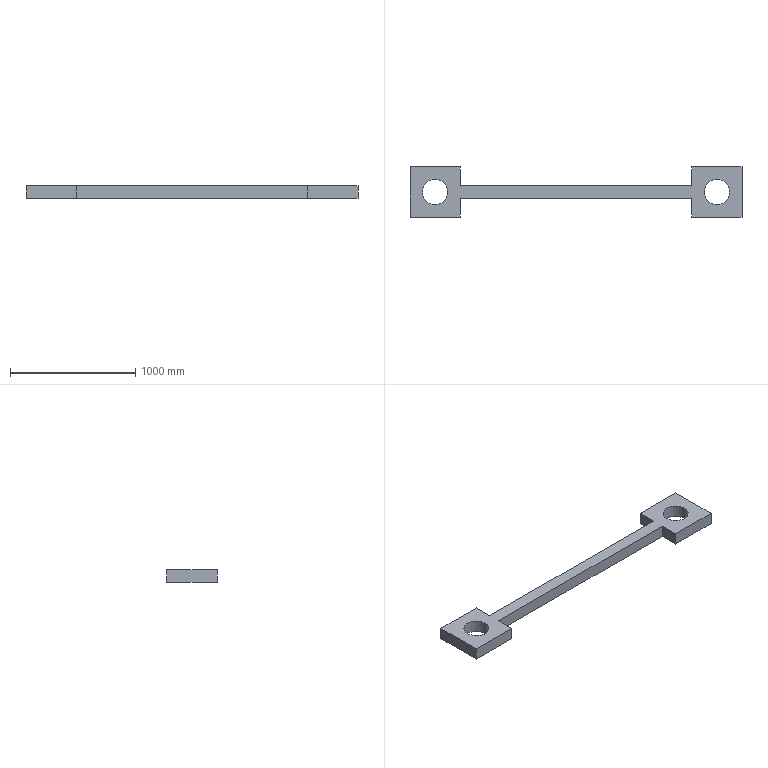Part | SolidWorks | features Extrusion 1 | 1 solid | 18 faces | box 2650 x 400 x 100 mm | volume 44216815 mm3 | plane 14 | cylinder 4 | commonest cylinder face diameters 200 x4
STEP:
#1=CARTESIAN_POINT('',(2150.,0.,100.));
#2=VERTEX_POINT('',#1);
#3=CARTESIAN_POINT('',(2350.,0.,100.));
#4=VERTEX_POINT('',#3);
#5=CARTESIAN_POINT('',(2250.,0.,100.));
#6=DIRECTION('',(0.,0.,1.));
#7=DIRECTION('',(1.,0.,0.));
#8=AXIS2_PLACEMENT_3D('',#5,#6,#7);
#9=CIRCLE('',#8,100.);
#10=EDGE_CURVE('',#2,#4,#9,.T.);
#11=ORIENTED_EDGE('',*,*,#10,.T.);
#12=CARTESIAN_POINT('',(2350.,0.,0.));
#13=VERTEX_POINT('',#12);
#14=CARTESIAN_POINT('',(2350.,0.,100.));
#15=DIRECTION('',(0.,0.,-1.));
#16=VECTOR('',#15,1000.);
#17=LINE('',#14,#16);
#18=EDGE_CURVE('',#4,#13,#17,.T.);
#19=ORIENTED_EDGE('',*,*,#18,.T.);
#20=CARTESIAN_POINT('',(2150.,0.,0.));
#21=VERTEX_POINT('',#20);
#22=CARTESIAN_POINT('',(2250.,0.,0.));
#23=DIRECTION('',(0.,0.,1.));
#24=DIRECTION('',(1.,0.,0.));
#25=AXIS2_PLACEMENT_3D('',#22,#23,#24);
#26=CIRCLE('',#25,100.);
#27=EDGE_CURVE('',#21,#13,#26,.T.);
#28=ORIENTED_EDGE('',*,*,#27,.F.);
#29=CARTESIAN_POINT('',(2150.,0.,100.));
#30=DIRECTION('',(0.,0.,-1.));
#31=VECTOR('',#30,1000.);
#32=LINE('',#29,#31);
#33=EDGE_CURVE('',#2,#21,#32,.T.);
#34=ORIENTED_EDGE('',*,*,#33,.F.);
#35=EDGE_LOOP('',(#11,#19,#28,#34));
#36=FACE_OUTER_BOUND('',#35,.T.);
#37=CARTESIAN_POINT('',(2250.,0.,100.));
#38=DIRECTION('',(0.,0.,-1.));
#39=DIRECTION('',(-1.,0.,0.));
#40=AXIS2_PLACEMENT_3D('',#37,#38,#39);
#41=CYLINDRICAL_SURFACE('',#40,100.);
#42=ADVANCED_FACE('',(#36),#41,.F.);
#43=CARTESIAN_POINT('',(-100.,0.,100.));
#44=VERTEX_POINT('',#43);
#45=CARTESIAN_POINT('',(100.,0.,100.));
#46=VERTEX_POINT('',#45);
#47=CARTESIAN_POINT('',(0.,0.,100.));
#48=DIRECTION('',(0.,0.,1.));
#49=DIRECTION('',(1.,0.,0.));
#50=AXIS2_PLACEMENT_3D('',#47,#48,#49);
#51=CIRCLE('',#50,100.);
#52=EDGE_CURVE('',#44,#46,#51,.T.);
#53=ORIENTED_EDGE('',*,*,#52,.T.);
#54=CARTESIAN_POINT('',(100.,0.,0.));
#55=VERTEX_POINT('',#54);
#56=CARTESIAN_POINT('',(100.,0.,100.));
#57=DIRECTION('',(0.,0.,-1.));
#58=VECTOR('',#57,1000.);
#59=LINE('',#56,#58);
#60=EDGE_CURVE('',#46,#55,#59,.T.);
#61=ORIENTED_EDGE('',*,*,#60,.T.);
#62=CARTESIAN_POINT('',(-100.,0.,0.));
#63=VERTEX_POINT('',#62);
#64=CARTESIAN_POINT('',(0.,0.,0.));
#65=DIRECTION('',(0.,0.,1.));
#66=DIRECTION('',(1.,0.,0.));
#67=AXIS2_PLACEMENT_3D('',#64,#65,#66);
#68=CIRCLE('',#67,100.);
#69=EDGE_CURVE('',#63,#55,#68,.T.);
#70=ORIENTED_EDGE('',*,*,#69,.F.);
#71=CARTESIAN_POINT('',(-100.,0.,100.));
#72=DIRECTION('',(0.,0.,-1.));
#73=VECTOR('',#72,1000.);
#74=LINE('',#71,#73);
#75=EDGE_CURVE('',#44,#63,#74,.T.);
#76=ORIENTED_EDGE('',*,*,#75,.F.);
#77=EDGE_LOOP('',(#53,#61,#70,#76));
#78=FACE_OUTER_BOUND('',#77,.T.);
#79=CARTESIAN_POINT('',(0.,0.,100.));
#80=DIRECTION('',(0.,0.,-1.));
#81=DIRECTION('',(-1.,0.,0.));
#82=AXIS2_PLACEMENT_3D('',#79,#80,#81);
#83=CYLINDRICAL_SURFACE('',#82,100.);
#84=ADVANCED_FACE('',(#78),#83,.F.);
#85=ORIENTED_EDGE('',*,*,#52,.F.);
#86=CARTESIAN_POINT('',(0.,0.,100.));
#87=DIRECTION('',(0.,0.,1.));
#88=DIRECTION('',(1.,0.,0.));
#89=AXIS2_PLACEMENT_3D('',#86,#87,#88);
#90=CIRCLE('',#89,100.);
#91=EDGE_CURVE('',#46,#44,#90,.T.);
#92=ORIENTED_EDGE('',*,*,#91,.F.);
#93=EDGE_LOOP('',(#85,#92));
#94=FACE_BOUND('',#93,.T.);
#95=CARTESIAN_POINT('',(-200.,200.,100.));
#96=VERTEX_POINT('',#95);
#97=CARTESIAN_POINT('',(-200.,-200.,100.));
#98=VERTEX_POINT('',#97);
#99=CARTESIAN_POINT('',(-200.,200.,100.));
#100=DIRECTION('',(0.,-1.,0.));
#101=VECTOR('',#100,1000.);
#102=LINE('',#99,#101);
#103=EDGE_CURVE('',#96,#98,#102,.T.);
#104=ORIENTED_EDGE('',*,*,#103,.T.);
#105=CARTESIAN_POINT('',(200.,-200.,100.));
#106=VERTEX_POINT('',#105);
#107=CARTESIAN_POINT('',(-200.,-200.,100.));
#108=DIRECTION('',(1.,0.,0.));
#109=VECTOR('',#108,1000.);
#110=LINE('',#107,#109);
#111=EDGE_CURVE('',#98,#106,#110,.T.);
#112=ORIENTED_EDGE('',*,*,#111,.T.);
#113=CARTESIAN_POINT('',(200.,-50.,100.));
#114=VERTEX_POINT('',#113);
#115=CARTESIAN_POINT('',(200.,-50.,100.));
#116=DIRECTION('',(0.,1.,0.));
#117=VECTOR('',#116,1000.);
#118=LINE('',#115,#117);
#119=EDGE_CURVE('',#106,#114,#118,.T.);
#120=ORIENTED_EDGE('',*,*,#119,.T.);
#121=CARTESIAN_POINT('',(2050.,-50.,100.));
#122=VERTEX_POINT('',#121);
#123=CARTESIAN_POINT('',(200.,-50.,100.));
#124=DIRECTION('',(1.,0.,0.));
#125=VECTOR('',#124,1000.);
#126=LINE('',#123,#125);
#127=EDGE_CURVE('',#114,#122,#126,.T.);
#128=ORIENTED_EDGE('',*,*,#127,.T.);
#129=CARTESIAN_POINT('',(2050.,-200.,100.));
#130=VERTEX_POINT('',#129);
#131=CARTESIAN_POINT('',(2050.,-50.,100.));
#132=DIRECTION('',(0.,-1.,0.));
#133=VECTOR('',#132,1000.);
#134=LINE('',#131,#133);
#135=EDGE_CURVE('',#122,#130,#134,.T.);
#136=ORIENTED_EDGE('',*,*,#135,.T.);
#137=CARTESIAN_POINT('',(2450.,-200.,100.));
#138=VERTEX_POINT('',#137);
#139=CARTESIAN_POINT('',(2050.,-200.,100.));
#140=DIRECTION('',(1.,0.,0.));
#141=VECTOR('',#140,1000.);
#142=LINE('',#139,#141);
#143=EDGE_CURVE('',#130,#138,#142,.T.);
#144=ORIENTED_EDGE('',*,*,#143,.T.);
#145=CARTESIAN_POINT('',(2450.,200.,100.));
#146=VERTEX_POINT('',#145);
#147=CARTESIAN_POINT('',(2450.,200.,100.));
#148=DIRECTION('',(0.,1.,0.));
#149=VECTOR('',#148,1000.);
#150=LINE('',#147,#149);
#151=EDGE_CURVE('',#138,#146,#150,.T.);
#152=ORIENTED_EDGE('',*,*,#151,.T.);
#153=CARTESIAN_POINT('',(2050.,200.,100.));
#154=VERTEX_POINT('',#153);
#155=CARTESIAN_POINT('',(2050.,200.,100.));
#156=DIRECTION('',(-1.,0.,0.));
#157=VECTOR('',#156,1000.);
#158=LINE('',#155,#157);
#159=EDGE_CURVE('',#146,#154,#158,.T.);
#160=ORIENTED_EDGE('',*,*,#159,.T.);
#161=CARTESIAN_POINT('',(2050.,50.,100.));
#162=VERTEX_POINT('',#161);
#163=CARTESIAN_POINT('',(2050.,200.,100.));
#164=DIRECTION('',(0.,-1.,0.));
#165=VECTOR('',#164,1000.);
#166=LINE('',#163,#165);
#167=EDGE_CURVE('',#154,#162,#166,.T.);
#168=ORIENTED_EDGE('',*,*,#167,.T.);
#169=CARTESIAN_POINT('',(200.,50.,100.));
#170=VERTEX_POINT('',#169);
#171=CARTESIAN_POINT('',(200.,50.,100.));
#172=DIRECTION('',(-1.,0.,0.));
#173=VECTOR('',#172,1000.);
#174=LINE('',#171,#173);
#175=EDGE_CURVE('',#162,#170,#174,.T.);
#176=ORIENTED_EDGE('',*,*,#175,.T.);
#177=CARTESIAN_POINT('',(200.,200.,100.));
#178=VERTEX_POINT('',#177);
#179=CARTESIAN_POINT('',(200.,200.,100.));
#180=DIRECTION('',(0.,1.,0.));
#181=VECTOR('',#180,1000.);
#182=LINE('',#179,#181);
#183=EDGE_CURVE('',#170,#178,#182,.T.);
#184=ORIENTED_EDGE('',*,*,#183,.T.);
#185=CARTESIAN_POINT('',(-200.,200.,100.));
#186=DIRECTION('',(-1.,0.,0.));
#187=VECTOR('',#186,1000.);
#188=LINE('',#185,#187);
#189=EDGE_CURVE('',#178,#96,#188,.T.);
#190=ORIENTED_EDGE('',*,*,#189,.T.);
#191=EDGE_LOOP('',(#104,#112,#120,#128,#136,#144,#152,#160,#168,#176,#184,#190));
#192=FACE_OUTER_BOUND('',#191,.T.);
#193=ORIENTED_EDGE('',*,*,#10,.F.);
#194=CARTESIAN_POINT('',(2250.,0.,100.));
#195=DIRECTION('',(0.,0.,1.));
#196=DIRECTION('',(1.,0.,0.));
#197=AXIS2_PLACEMENT_3D('',#194,#195,#196);
#198=CIRCLE('',#197,100.);
#199=EDGE_CURVE('',#4,#2,#198,.T.);
#200=ORIENTED_EDGE('',*,*,#199,.F.);
#201=EDGE_LOOP('',(#193,#200));
#202=FACE_BOUND('',#201,.T.);
#203=CARTESIAN_POINT('',(-200.,-200.,100.));
#204=DIRECTION('',(0.,0.,1.));
#205=DIRECTION('',(1.,0.,0.));
#206=AXIS2_PLACEMENT_3D('',#203,#204,#205);
#207=PLANE('',#206);
#208=ADVANCED_FACE('',(#94,#192,#202),#207,.T.);
#209=ORIENTED_EDGE('',*,*,#69,.T.);
#210=CARTESIAN_POINT('',(0.,0.,0.));
#211=DIRECTION('',(0.,0.,1.));
#212=DIRECTION('',(1.,0.,0.));
#213=AXIS2_PLACEMENT_3D('',#210,#211,#212);
#214=CIRCLE('',#213,100.);
#215=EDGE_CURVE('',#55,#63,#214,.T.);
#216=ORIENTED_EDGE('',*,*,#215,.T.);
#217=EDGE_LOOP('',(#209,#216));
#218=FACE_BOUND('',#217,.T.);
#219=CARTESIAN_POINT('',(-200.,200.,0.));
#220=VERTEX_POINT('',#219);
#221=CARTESIAN_POINT('',(-200.,-200.,0.));
#222=VERTEX_POINT('',#221);
#223=CARTESIAN_POINT('',(-200.,200.,0.));
#224=DIRECTION('',(0.,-1.,0.));
#225=VECTOR('',#224,1000.);
#226=LINE('',#223,#225);
#227=EDGE_CURVE('',#220,#222,#226,.T.);
#228=ORIENTED_EDGE('',*,*,#227,.F.);
#229=CARTESIAN_POINT('',(200.,200.,0.));
#230=VERTEX_POINT('',#229);
#231=CARTESIAN_POINT('',(-200.,200.,0.));
#232=DIRECTION('',(-1.,0.,0.));
#233=VECTOR('',#232,1000.);
#234=LINE('',#231,#233);
#235=EDGE_CURVE('',#230,#220,#234,.T.);
#236=ORIENTED_EDGE('',*,*,#235,.F.);
#237=CARTESIAN_POINT('',(200.,50.,0.));
#238=VERTEX_POINT('',#237);
#239=CARTESIAN_POINT('',(200.,200.,0.));
#240=DIRECTION('',(0.,1.,0.));
#241=VECTOR('',#240,1000.);
#242=LINE('',#239,#241);
#243=EDGE_CURVE('',#238,#230,#242,.T.);
#244=ORIENTED_EDGE('',*,*,#243,.F.);
#245=CARTESIAN_POINT('',(2050.,50.,0.));
#246=VERTEX_POINT('',#245);
#247=CARTESIAN_POINT('',(200.,50.,0.));
#248=DIRECTION('',(-1.,0.,0.));
#249=VECTOR('',#248,1000.);
#250=LINE('',#247,#249);
#251=EDGE_CURVE('',#246,#238,#250,.T.);
#252=ORIENTED_EDGE('',*,*,#251,.F.);
#253=CARTESIAN_POINT('',(2050.,200.,0.));
#254=VERTEX_POINT('',#253);
#255=CARTESIAN_POINT('',(2050.,200.,0.));
#256=DIRECTION('',(0.,-1.,0.));
#257=VECTOR('',#256,1000.);
#258=LINE('',#255,#257);
#259=EDGE_CURVE('',#254,#246,#258,.T.);
#260=ORIENTED_EDGE('',*,*,#259,.F.);
#261=CARTESIAN_POINT('',(2450.,200.,0.));
#262=VERTEX_POINT('',#261);
#263=CARTESIAN_POINT('',(2050.,200.,0.));
#264=DIRECTION('',(-1.,0.,0.));
#265=VECTOR('',#264,1000.);
#266=LINE('',#263,#265);
#267=EDGE_CURVE('',#262,#254,#266,.T.);
#268=ORIENTED_EDGE('',*,*,#267,.F.);
#269=CARTESIAN_POINT('',(2450.,-200.,0.));
#270=VERTEX_POINT('',#269);
#271=CARTESIAN_POINT('',(2450.,200.,0.));
#272=DIRECTION('',(0.,1.,0.));
#273=VECTOR('',#272,1000.);
#274=LINE('',#271,#273);
#275=EDGE_CURVE('',#270,#262,#274,.T.);
#276=ORIENTED_EDGE('',*,*,#275,.F.);
#277=CARTESIAN_POINT('',(2050.,-200.,0.));
#278=VERTEX_POINT('',#277);
#279=CARTESIAN_POINT('',(2050.,-200.,0.));
#280=DIRECTION('',(1.,0.,0.));
#281=VECTOR('',#280,1000.);
#282=LINE('',#279,#281);
#283=EDGE_CURVE('',#278,#270,#282,.T.);
#284=ORIENTED_EDGE('',*,*,#283,.F.);
#285=CARTESIAN_POINT('',(2050.,-50.,0.));
#286=VERTEX_POINT('',#285);
#287=CARTESIAN_POINT('',(2050.,-50.,0.));
#288=DIRECTION('',(0.,-1.,0.));
#289=VECTOR('',#288,1000.);
#290=LINE('',#287,#289);
#291=EDGE_CURVE('',#286,#278,#290,.T.);
#292=ORIENTED_EDGE('',*,*,#291,.F.);
#293=CARTESIAN_POINT('',(200.,-50.,0.));
#294=VERTEX_POINT('',#293);
#295=CARTESIAN_POINT('',(200.,-50.,0.));
#296=DIRECTION('',(1.,0.,0.));
#297=VECTOR('',#296,1000.);
#298=LINE('',#295,#297);
#299=EDGE_CURVE('',#294,#286,#298,.T.);
#300=ORIENTED_EDGE('',*,*,#299,.F.);
#301=CARTESIAN_POINT('',(200.,-200.,0.));
#302=VERTEX_POINT('',#301);
#303=CARTESIAN_POINT('',(200.,-50.,0.));
#304=DIRECTION('',(0.,1.,0.));
#305=VECTOR('',#304,1000.);
#306=LINE('',#303,#305);
#307=EDGE_CURVE('',#302,#294,#306,.T.);
#308=ORIENTED_EDGE('',*,*,#307,.F.);
#309=CARTESIAN_POINT('',(-200.,-200.,0.));
#310=DIRECTION('',(1.,0.,0.));
#311=VECTOR('',#310,1000.);
#312=LINE('',#309,#311);
#313=EDGE_CURVE('',#222,#302,#312,.T.);
#314=ORIENTED_EDGE('',*,*,#313,.F.);
#315=EDGE_LOOP('',(#228,#236,#244,#252,#260,#268,#276,#284,#292,#300,#308,#314));
#316=FACE_OUTER_BOUND('',#315,.T.);
#317=ORIENTED_EDGE('',*,*,#27,.T.);
#318=CARTESIAN_POINT('',(2250.,0.,0.));
#319=DIRECTION('',(0.,0.,1.));
#320=DIRECTION('',(1.,0.,0.));
#321=AXIS2_PLACEMENT_3D('',#318,#319,#320);
#322=CIRCLE('',#321,100.);
#323=EDGE_CURVE('',#13,#21,#322,.T.);
#324=ORIENTED_EDGE('',*,*,#323,.T.);
#325=EDGE_LOOP('',(#317,#324));
#326=FACE_BOUND('',#325,.T.);
#327=CARTESIAN_POINT('',(-200.,-200.,0.));
#328=DIRECTION('',(0.,0.,1.));
#329=DIRECTION('',(1.,0.,0.));
#330=AXIS2_PLACEMENT_3D('',#327,#328,#329);
#331=PLANE('',#330);
#332=ADVANCED_FACE('',(#218,#316,#326),#331,.F.);
#333=ORIENTED_EDGE('',*,*,#227,.T.);
#334=CARTESIAN_POINT('',(-200.,-200.,100.));
#335=DIRECTION('',(0.,0.,-1.));
#336=VECTOR('',#335,1000.);
#337=LINE('',#334,#336);
#338=EDGE_CURVE('',#98,#222,#337,.T.);
#339=ORIENTED_EDGE('',*,*,#338,.F.);
#340=ORIENTED_EDGE('',*,*,#103,.F.);
#341=CARTESIAN_POINT('',(-200.,200.,100.));
#342=DIRECTION('',(0.,0.,-1.));
#343=VECTOR('',#342,1000.);
#344=LINE('',#341,#343);
#345=EDGE_CURVE('',#96,#220,#344,.T.);
#346=ORIENTED_EDGE('',*,*,#345,.T.);
#347=EDGE_LOOP('',(#333,#339,#340,#346));
#348=FACE_OUTER_BOUND('',#347,.T.);
#349=CARTESIAN_POINT('',(-200.,200.,100.));
#350=DIRECTION('',(1.,0.,0.));
#351=DIRECTION('',(0.,1.,0.));
#352=AXIS2_PLACEMENT_3D('',#349,#350,#351);
#353=PLANE('',#352);
#354=ADVANCED_FACE('',(#348),#353,.F.);
#355=ORIENTED_EDGE('',*,*,#313,.T.);
#356=CARTESIAN_POINT('',(200.,-200.,100.));
#357=DIRECTION('',(0.,0.,-1.));
#358=VECTOR('',#357,1000.);
#359=LINE('',#356,#358);
#360=EDGE_CURVE('',#106,#302,#359,.T.);
#361=ORIENTED_EDGE('',*,*,#360,.F.);
#362=ORIENTED_EDGE('',*,*,#111,.F.);
#363=ORIENTED_EDGE('',*,*,#338,.T.);
#364=EDGE_LOOP('',(#355,#361,#362,#363));
#365=FACE_OUTER_BOUND('',#364,.T.);
#366=CARTESIAN_POINT('',(-200.,-200.,100.));
#367=DIRECTION('',(0.,1.,0.));
#368=DIRECTION('',(-1.,0.,0.));
#369=AXIS2_PLACEMENT_3D('',#366,#367,#368);
#370=PLANE('',#369);
#371=ADVANCED_FACE('',(#365),#370,.F.);
#372=ORIENTED_EDGE('',*,*,#307,.T.);
#373=CARTESIAN_POINT('',(200.,-50.,100.));
#374=DIRECTION('',(0.,0.,-1.));
#375=VECTOR('',#374,1000.);
#376=LINE('',#373,#375);
#377=EDGE_CURVE('',#114,#294,#376,.T.);
#378=ORIENTED_EDGE('',*,*,#377,.F.);
#379=ORIENTED_EDGE('',*,*,#119,.F.);
#380=ORIENTED_EDGE('',*,*,#360,.T.);
#381=EDGE_LOOP('',(#372,#378,#379,#380));
#382=FACE_OUTER_BOUND('',#381,.T.);
#383=CARTESIAN_POINT('',(200.,-50.,100.));
#384=DIRECTION('',(-1.,0.,0.));
#385=DIRECTION('',(0.,0.,1.));
#386=AXIS2_PLACEMENT_3D('',#383,#384,#385);
#387=PLANE('',#386);
#388=ADVANCED_FACE('',(#382),#387,.F.);
#389=ORIENTED_EDGE('',*,*,#299,.T.);
#390=CARTESIAN_POINT('',(2050.,-50.,100.));
#391=DIRECTION('',(0.,0.,-1.));
#392=VECTOR('',#391,1000.);
#393=LINE('',#390,#392);
#394=EDGE_CURVE('',#122,#286,#393,.T.);
#395=ORIENTED_EDGE('',*,*,#394,.F.);
#396=ORIENTED_EDGE('',*,*,#127,.F.);
#397=ORIENTED_EDGE('',*,*,#377,.T.);
#398=EDGE_LOOP('',(#389,#395,#396,#397));
#399=FACE_OUTER_BOUND('',#398,.T.);
#400=CARTESIAN_POINT('',(200.,-50.,100.));
#401=DIRECTION('',(0.,1.,0.));
#402=DIRECTION('',(0.,0.,1.));
#403=AXIS2_PLACEMENT_3D('',#400,#401,#402);
#404=PLANE('',#403);
#405=ADVANCED_FACE('',(#399),#404,.F.);
#406=ORIENTED_EDGE('',*,*,#291,.T.);
#407=CARTESIAN_POINT('',(2050.,-200.,100.));
#408=DIRECTION('',(0.,0.,-1.));
#409=VECTOR('',#408,1000.);
#410=LINE('',#407,#409);
#411=EDGE_CURVE('',#130,#278,#410,.T.);
#412=ORIENTED_EDGE('',*,*,#411,.F.);
#413=ORIENTED_EDGE('',*,*,#135,.F.);
#414=ORIENTED_EDGE('',*,*,#394,.T.);
#415=EDGE_LOOP('',(#406,#412,#413,#414));
#416=FACE_OUTER_BOUND('',#415,.T.);
#417=CARTESIAN_POINT('',(2050.,-50.,100.));
#418=DIRECTION('',(1.,0.,0.));
#419=DIRECTION('',(0.,0.,-1.));
#420=AXIS2_PLACEMENT_3D('',#417,#418,#419);
#421=PLANE('',#420);
#422=ADVANCED_FACE('',(#416),#421,.F.);
#423=ORIENTED_EDGE('',*,*,#283,.T.);
#424=CARTESIAN_POINT('',(2450.,-200.,100.));
#425=DIRECTION('',(0.,0.,-1.));
#426=VECTOR('',#425,1000.);
#427=LINE('',#424,#426);
#428=EDGE_CURVE('',#138,#270,#427,.T.);
#429=ORIENTED_EDGE('',*,*,#428,.F.);
#430=ORIENTED_EDGE('',*,*,#143,.F.);
#431=ORIENTED_EDGE('',*,*,#411,.T.);
#432=EDGE_LOOP('',(#423,#429,#430,#431));
#433=FACE_OUTER_BOUND('',#432,.T.);
#434=CARTESIAN_POINT('',(2050.,-200.,100.));
#435=DIRECTION('',(0.,1.,0.));
#436=DIRECTION('',(-1.,0.,0.));
#437=AXIS2_PLACEMENT_3D('',#434,#435,#436);
#438=PLANE('',#437);
#439=ADVANCED_FACE('',(#433),#438,.F.);
#440=ORIENTED_EDGE('',*,*,#275,.T.);
#441=CARTESIAN_POINT('',(2450.,200.,100.));
#442=DIRECTION('',(0.,0.,-1.));
#443=VECTOR('',#442,1000.);
#444=LINE('',#441,#443);
#445=EDGE_CURVE('',#146,#262,#444,.T.);
#446=ORIENTED_EDGE('',*,*,#445,.F.);
#447=ORIENTED_EDGE('',*,*,#151,.F.);
#448=ORIENTED_EDGE('',*,*,#428,.T.);
#449=EDGE_LOOP('',(#440,#446,#447,#448));
#450=FACE_OUTER_BOUND('',#449,.T.);
#451=CARTESIAN_POINT('',(2450.,200.,100.));
#452=DIRECTION('',(-1.,0.,0.));
#453=DIRECTION('',(0.,0.,1.));
#454=AXIS2_PLACEMENT_3D('',#451,#452,#453);
#455=PLANE('',#454);
#456=ADVANCED_FACE('',(#450),#455,.F.);
#457=ORIENTED_EDGE('',*,*,#267,.T.);
#458=CARTESIAN_POINT('',(2050.,200.,100.));
#459=DIRECTION('',(0.,0.,-1.));
#460=VECTOR('',#459,1000.);
#461=LINE('',#458,#460);
#462=EDGE_CURVE('',#154,#254,#461,.T.);
#463=ORIENTED_EDGE('',*,*,#462,.F.);
#464=ORIENTED_EDGE('',*,*,#159,.F.);
#465=ORIENTED_EDGE('',*,*,#445,.T.);
#466=EDGE_LOOP('',(#457,#463,#464,#465));
#467=FACE_OUTER_BOUND('',#466,.T.);
#468=CARTESIAN_POINT('',(2050.,200.,100.));
#469=DIRECTION('',(0.,-1.,0.));
#470=DIRECTION('',(1.,0.,0.));
#471=AXIS2_PLACEMENT_3D('',#468,#469,#470);
#472=PLANE('',#471);
#473=ADVANCED_FACE('',(#467),#472,.F.);
#474=ORIENTED_EDGE('',*,*,#259,.T.);
#475=CARTESIAN_POINT('',(2050.,50.,100.));
#476=DIRECTION('',(0.,0.,-1.));
#477=VECTOR('',#476,1000.);
#478=LINE('',#475,#477);
#479=EDGE_CURVE('',#162,#246,#478,.T.);
#480=ORIENTED_EDGE('',*,*,#479,.F.);
#481=ORIENTED_EDGE('',*,*,#167,.F.);
#482=ORIENTED_EDGE('',*,*,#462,.T.);
#483=EDGE_LOOP('',(#474,#480,#481,#482));
#484=FACE_OUTER_BOUND('',#483,.T.);
#485=CARTESIAN_POINT('',(2050.,200.,100.));
#486=DIRECTION('',(1.,0.,0.));
#487=DIRECTION('',(0.,0.,-1.));
#488=AXIS2_PLACEMENT_3D('',#485,#486,#487);
#489=PLANE('',#488);
#490=ADVANCED_FACE('',(#484),#489,.F.);
#491=ORIENTED_EDGE('',*,*,#251,.T.);
#492=CARTESIAN_POINT('',(200.,50.,100.));
#493=DIRECTION('',(0.,0.,-1.));
#494=VECTOR('',#493,1000.);
#495=LINE('',#492,#494);
#496=EDGE_CURVE('',#170,#238,#495,.T.);
#497=ORIENTED_EDGE('',*,*,#496,.F.);
#498=ORIENTED_EDGE('',*,*,#175,.F.);
#499=ORIENTED_EDGE('',*,*,#479,.T.);
#500=EDGE_LOOP('',(#491,#497,#498,#499));
#501=FACE_OUTER_BOUND('',#500,.T.);
#502=CARTESIAN_POINT('',(200.,50.,100.));
#503=DIRECTION('',(0.,-1.,0.));
#504=DIRECTION('',(0.,0.,-1.));
#505=AXIS2_PLACEMENT_3D('',#502,#503,#504);
#506=PLANE('',#505);
#507=ADVANCED_FACE('',(#501),#506,.F.);
#508=ORIENTED_EDGE('',*,*,#243,.T.);
#509=CARTESIAN_POINT('',(200.,200.,100.));
#510=DIRECTION('',(0.,0.,-1.));
#511=VECTOR('',#510,1000.);
#512=LINE('',#509,#511);
#513=EDGE_CURVE('',#178,#230,#512,.T.);
#514=ORIENTED_EDGE('',*,*,#513,.F.);
#515=ORIENTED_EDGE('',*,*,#183,.F.);
#516=ORIENTED_EDGE('',*,*,#496,.T.);
#517=EDGE_LOOP('',(#508,#514,#515,#516));
#518=FACE_OUTER_BOUND('',#517,.T.);
#519=CARTESIAN_POINT('',(200.,200.,100.));
#520=DIRECTION('',(-1.,0.,0.));
#521=DIRECTION('',(0.,-1.,0.));
#522=AXIS2_PLACEMENT_3D('',#519,#520,#521);
#523=PLANE('',#522);
#524=ADVANCED_FACE('',(#518),#523,.F.);
#525=ORIENTED_EDGE('',*,*,#235,.T.);
#526=ORIENTED_EDGE('',*,*,#345,.F.);
#527=ORIENTED_EDGE('',*,*,#189,.F.);
#528=ORIENTED_EDGE('',*,*,#513,.T.);
#529=EDGE_LOOP('',(#525,#526,#527,#528));
#530=FACE_OUTER_BOUND('',#529,.T.);
#531=CARTESIAN_POINT('',(-200.,200.,100.));
#532=DIRECTION('',(0.,-1.,0.));
#533=DIRECTION('',(0.,0.,-1.));
#534=AXIS2_PLACEMENT_3D('',#531,#532,#533);
#535=PLANE('',#534);
#536=ADVANCED_FACE('',(#530),#535,.F.);
#537=ORIENTED_EDGE('',*,*,#60,.F.);
#538=ORIENTED_EDGE('',*,*,#91,.T.);
#539=ORIENTED_EDGE('',*,*,#75,.T.);
#540=ORIENTED_EDGE('',*,*,#215,.F.);
#541=EDGE_LOOP('',(#537,#538,#539,#540));
#542=FACE_OUTER_BOUND('',#541,.T.);
#543=CARTESIAN_POINT('',(0.,0.,100.));
#544=DIRECTION('',(0.,0.,-1.));
#545=DIRECTION('',(-1.,0.,0.));
#546=AXIS2_PLACEMENT_3D('',#543,#544,#545);
#547=CYLINDRICAL_SURFACE('',#546,100.);
#548=ADVANCED_FACE('',(#542),#547,.F.);
#549=ORIENTED_EDGE('',*,*,#18,.F.);
#550=ORIENTED_EDGE('',*,*,#199,.T.);
#551=ORIENTED_EDGE('',*,*,#33,.T.);
#552=ORIENTED_EDGE('',*,*,#323,.F.);
#553=EDGE_LOOP('',(#549,#550,#551,#552));
#554=FACE_OUTER_BOUND('',#553,.T.);
#555=CARTESIAN_POINT('',(2250.,0.,100.));
#556=DIRECTION('',(0.,0.,-1.));
#557=DIRECTION('',(-1.,0.,0.));
#558=AXIS2_PLACEMENT_3D('',#555,#556,#557);
#559=CYLINDRICAL_SURFACE('',#558,100.);
#560=ADVANCED_FACE('',(#554),#559,.F.);
#561=CLOSED_SHELL('',(#42,#84,#208,#332,#354,#371,#388,#405,#422,#439,#456,#473,#490,#507,#524,#536,#548,#560));
#562=MANIFOLD_SOLID_BREP('',#561);
#563=CARTESIAN_POINT('',(0.,0.,0.));
#564=DIRECTION('',(0.,0.,1.));
#565=DIRECTION('',(1.,0.,0.));
#566=AXIS2_PLACEMENT_3D('',#563,#564,#565);
#567=(LENGTH_UNIT()NAMED_UNIT(*)SI_UNIT(.MILLI.,.METRE.));
#568=UNCERTAINTY_MEASURE_WITH_UNIT(LENGTH_MEASURE(0.00001),#567,'','');
#569=(NAMED_UNIT(*)PLANE_ANGLE_UNIT()SI_UNIT($,.RADIAN.));
#570=(NAMED_UNIT(*)SI_UNIT($,.STERADIAN.)SOLID_ANGLE_UNIT());
#571=(GEOMETRIC_REPRESENTATION_CONTEXT(3)GLOBAL_UNCERTAINTY_ASSIGNED_CONTEXT((#568))GLOBAL_UNIT_ASSIGNED_CONTEXT((#567,#569,#570))REPRESENTATION_CONTEXT('',''));
#572=ADVANCED_BREP_SHAPE_REPRESENTATION('',(#562,#566),#571);